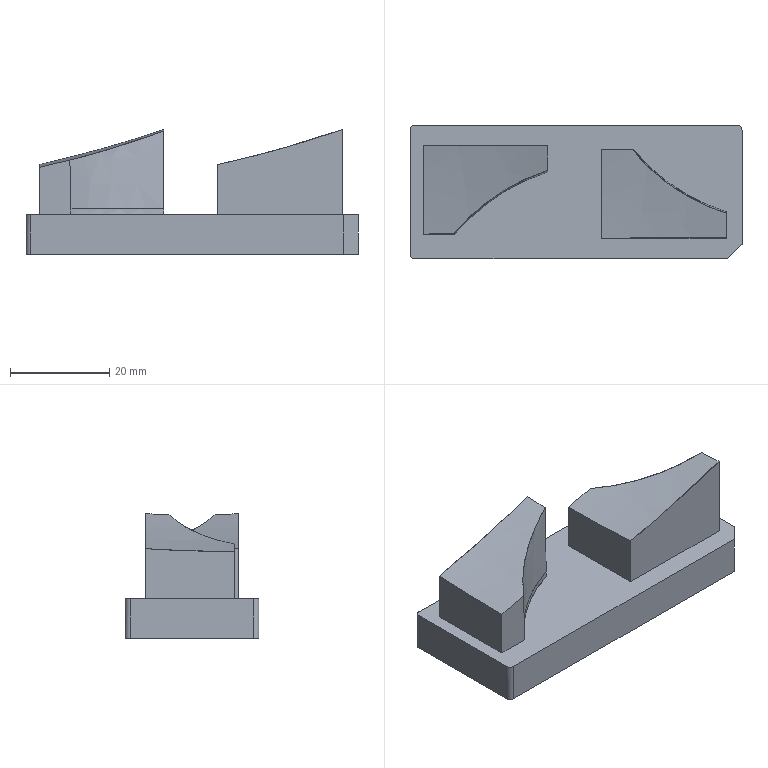NC program | PowerMill | posted with a generic post | part box 67 x 27 x 25.167 mm
Lines 9936 to 10890 of 102458:
N10033 M6
N10034 S18000 M03
N10035 G00 G90 X0.0 Y0.0
N10036 G43 Z9.797 H2
N10037
N10038 G05 P10000 R4
N10039 X-5.4152 Y3.5784
N10040 Z0.7883
N10041 G01 Z-0.4117 F3600.0
N10042 X-5.4161 Y3.6004 F6000.0
N10043 G03 X-5.6216 Y3.7906 I-0.1978 J-0.0077
N10044 G01 X-5.8566 Y3.7814
N10045 X-6.3615 Y3.9044
N10046 X-6.8327 Y4.1332
N10047 X-7.1219 Y4.3925
N10048 X-7.3208 Y4.6168
N10049 X-7.4743 Y4.8805
N10050 X-7.6448 Y5.3686
N10051 X-7.7024 Y5.8566
N10052 X-8.2969 Y8.9999
N10053 X-8.3233 Y9.273
N10054 X-8.2722 Y9.7611
N10055 X-8.0896 Y10.2491
N10056 X-7.725 Y10.7372
N10057 X-7.3208 Y11.0423
N10058 X-6.9004 Y11.2252
N10059 X-6.3447 Y11.3099
N10060 X-5.3686 Y11.2842
N10061 X-5.1132 Y11.2252
N10062 X-4.8805 Y11.139
N10063 X-4.3925 Y10.8322
N10064 X-4.2886 Y10.7372
N10065 X-3.924 Y10.2491
N10066 X-3.7414 Y9.7611
N10067 X-3.6896 Y9.273
N10068 X-3.6899 Y5.8566
N10069 X-3.7357 Y5.3686
N10070 X-3.9016 Y4.8805
N10071 X-4.2608 Y4.3925
N10072 X-4.3925 Y4.253
N10073 X-4.8805 Y3.9455
N10074 X-5.014 Y3.9044
N10075 X-5.2381 Y3.8387
N10076 G00 Z3.5896
N10077 G01 X-2.8266 Y3.5215 F10000.0
N10078 G00 Z0.5896
N10079 G01 Z-0.6104 F3600.0
N10080 X-2.8369 Y3.5409 F6000.0
N10081 G03 X-3.1046 Y3.6229 I-0.1749 J-0.0928
N10082 G01 X-4.1535 Y3.066
N10083 X-4.2516 Y2.9283
N10084 X-4.3925 Y2.7945
N10085 X-4.8805 Y2.4886
N10086 X-4.998 Y2.4403
N10087 X-5.3686 Y2.3172
N10088 X-5.8566 Y2.2169
N10089 X-6.3447 Y2.2398
N10090 X-6.8327 Y2.3884
N10091 X-7.3208 Y2.6994
N10092 X-7.543 Y2.9283
N10093 X-7.8088 Y3.3417
N10094 X-7.9847 Y3.9044
N10095 X-8.3032 Y5.8566
N10096 X-8.3036 Y5.8588
N10097 X-8.7849 Y8.4482
N10098 X-8.9269 Y9.273
N10099 X-8.8758 Y9.7611
N10100 X-8.7849 Y10.0479
N10101 X-8.6931 Y10.2491
N10102 X-8.3286 Y10.7372
N10103 X-7.8088 Y11.1036
N10104 X-7.504 Y11.2252
N10105 X-7.3208 Y11.2711
N10106 X-6.8327 Y11.3101
N10107 X-5.8566
N10108 X-5.3686 Y11.2842
N10109 X-5.1132 Y11.2252
N10110 X-4.8805 Y11.1391
N10111 X-4.3925 Y10.8322
N10112 X-4.2886 Y10.7372
N10113 X-3.924 Y10.2491
N10114 X-3.7414 Y9.7611
N10115 X-3.6896 Y9.273
N10116 X-3.6899 Y4.3925
N10117 X-3.7336 Y3.9044
N10118 X-3.9039 Y3.4164
N10119 X-4.1535 Y3.066
N10120 X-2.8242 Y3.5261 Z-0.8091
N10121 X-2.8346 Y3.5455
N10122 G03 X-3.1027 Y3.6263 I-0.1745 J-0.0936
N10123 G01 X-4.1508 Y3.0641
N10124 X-4.2467 Y2.9283
N10125 X-4.3925 Y2.7908
N10126 X-4.8805 Y2.4842
N10127 X-4.9878 Y2.4403
N10128 X-5.8566 Y2.1507
N10129 X-6.3447 Y2.0339
N10130 X-6.8327 Y2.0366
N10131 X-7.3208 Y2.1646
N10132 X-7.8024 Y2.4403
N10133 X-8.25 Y2.9283
N10134 X-8.481 Y3.4164
N10135 X-8.5847 Y3.9044
N10136 X-8.9074 Y5.8566
N10137 X-9.4613 Y8.7849
N10138 X-9.5304 Y9.273
N10139 X-9.4793 Y9.7611
N10140 X-9.2967 Y10.2491
N10141 X-8.9321 Y10.7372
N10142 X-8.7849 Y10.8677
N10143 X-8.2969 Y11.1564
N10144 X-8.1076 Y11.2252
N10145 X-7.8088 Y11.2903
N10146 X-6.974 Y11.2988
N10147 X-6.9672 Y11.2993
N10148 X-6.8327 Y11.3101
N10149 X-5.8617 Y11.31
N10150 X-5.8566 Y11.3101
N10151 X-5.3686 Y11.2842
N10152 X-5.1132 Y11.2252
N10153 X-4.8805 Y11.1391
N10154 X-4.3925 Y10.8322
N10155 X-4.2886 Y10.7372
N10156 X-3.924 Y10.2491
N10157 X-3.7414 Y9.7611
N10158 X-3.6896 Y9.273
N10159 X-3.6899 Y4.3925
N10160 X-3.7325 Y3.9044
N10161 X-3.9021 Y3.4164
N10162 X-4.1508 Y3.0641
N10163 X-2.8229 Y3.5279 Z-1.0077
N10164 X-2.8333 Y3.5472
N10165 G03 X-3.1016 Y3.6275 I-0.1743 J-0.094
N10166 G01 X-4.1488 Y3.0627
N10167 X-4.2432 Y2.9283
N10168 X-4.3925 Y2.7872
N10169 X-4.8805 Y2.4804
N10170 X-4.9342 Y2.4622
N10171 X-4.9878 Y2.4403
N10172 X-5.8567 Y2.1508
N10173 X-6.4447 Y1.9522
N10174 X-6.8327 Y1.852
N10175 X-7.3208 Y1.8346
N10176 X-7.8088 Y1.9405
N10177 X-8.2969 Y2.1945
N10178 X-8.5828 Y2.4403
N10179 X-8.7849 Y2.689
N10180 X-8.9299 Y2.9283
N10181 X-9.1003 Y3.4164
N10182 X-9.5117 Y5.8566
N10183 X-10.0649 Y8.7849
N10184 X-10.134 Y9.273
N10185 X-10.0829 Y9.7611
N10186 X-9.9003 Y10.2491
N10187 X-9.7611 Y10.4691
N10188 X-9.5357 Y10.7372
N10189 X-9.273 Y10.9512
N10190 X-8.7849 Y11.2013
N10191 X-8.2969 Y11.3032
N10192 X-6.8672 Y11.3072
N10193 X-6.8597 Y11.3079
N10194 X-6.8327 Y11.31
N10195 X-5.8929
N10196 X-5.8566 Y11.3101
N10197 X-5.3686 Y11.2842
N10198 X-5.1132 Y11.2252
N10199 X-4.8805 Y11.1391
N10200 X-4.3925 Y10.8322
N10201 X-4.2886 Y10.7372
N10202 X-3.924 Y10.2491
N10203 X-3.7414 Y9.7611
N10204 X-3.6896 Y9.273
N10205 X-3.6899 Y4.3925
N10206 X-3.7314 Y3.9044
N10207 X-3.9003 Y3.4164
N10208 X-4.1488 Y3.0627
N10209 X-2.8216 Y3.5296 Z-1.2064
N10210 X-2.8321 Y3.549
N10211 G03 X-3.1005 Y3.6286 I-0.174 J-0.0944
N10212 G01 X-4.1468 Y3.0613
N10213 X-4.2398 Y2.9283
N10214 X-4.3925 Y2.7836
N10215 X-4.8805 Y2.4767
N10216 X-4.9811 Y2.4428
N10217 X-4.9845 Y2.4416
N10218 X-4.9878 Y2.4404
N10219 X-5.018 Y2.4303
N10220 X-6.4332 Y1.9522
N10221 X-7.3208 Y1.6489
N10222 X-7.8088 Y1.611
N10223 X-8.2969 Y1.6947
N10224 X-8.7849 Y1.9191
N10225 X-9.273 Y2.3545
N10226 X-9.5969 Y2.9283
N10227 X-9.7102 Y3.4164
N10228 X-10.2931 Y6.8327
N10229 X-10.6685 Y8.7849
N10230 X-10.7376 Y9.273
N10231 X-10.6865 Y9.7611
N10232 X-10.5038 Y10.2491
N10233 X-10.2491 Y10.619
N10234 X-10.1393 Y10.7372
N10235 X-9.7611 Y11.0279
N10236 X-9.3147 Y11.2252
N10237 X-8.7849 Y11.3092
N10238 X-6.835 Y11.3098
N10239 X-6.8327 Y11.31
N10240 X-6.3069 Y11.3099
N10241 X-5.8566 Y11.3101
N10242 X-5.3686 Y11.2842
N10243 X-5.1132 Y11.2252
N10244 X-4.8805 Y11.1391
N10245 X-4.3925 Y10.8322
N10246 X-4.2886 Y10.7372
N10247 X-3.924 Y10.2491
N10248 X-3.7414 Y9.7611
N10249 X-3.6896 Y9.273
N10250 X-3.6899 Y4.3925
N10251 X-3.7305 Y3.9044
N10252 X-3.8985 Y3.4164
N10253 X-4.1468 Y3.0613
N10254 X-2.8223 Y3.5227 Z-1.4051
N10255 X-2.8328 Y3.5421
N10256 G03 X-3.1011 Y3.6223 I-0.1742 J-0.094
N10257 G01 X-4.1442 Y3.0594
N10258 X-4.2363 Y2.9283
N10259 X-4.3925 Y2.7799
N10260 X-4.8805 Y2.4731
N10261 X-6.3447 Y1.9781
N10262 X-7.7529 Y1.4642
N10263 X-8.2969 Y1.3898
N10264 X-8.7849 Y1.4526
N10265 X-9.273 Y1.6486
N10266 X-9.7611 Y2.0326
N10267 X-10.0491 Y2.4403
N10268 X-10.2376 Y2.9283
N10269 X-10.4718 Y4.3925
N10270 X-11.2252 Y8.5768
N10271 X-11.3411 Y9.273
N10272 X-11.29 Y9.7611
N10273 X-11.2252 Y9.9783
N10274 X-11.1074 Y10.2491
N10275 X-10.7372 Y10.7398
N10276 X-10.2491 Y11.0905
N10277 X-9.9183 Y11.2252
N10278 X-9.7611 Y11.2654
N10279 X-9.273 Y11.3101
N10280 X-5.8566
N10281 X-5.3686 Y11.2842
N10282 X-5.1132 Y11.2252
N10283 X-4.8805 Y11.1391
N10284 X-4.3925 Y10.8323
N10285 X-4.2886 Y10.7372
N10286 X-3.924 Y10.2491
N10287 X-3.7414 Y9.7611
N10288 X-3.6896 Y9.273
N10289 X-3.6899 Y4.3925
N10290 X-3.7298 Y3.9044
N10291 X-3.833 Y3.6069
N10292 X-3.8985 Y3.4164
N10293 X-3.9011 Y3.41
N10294 X-3.9035 Y3.4036
N10295 X-3.9044 Y3.4008
N10296 X-4.1442 Y3.0594
N10297 X-2.819 Y3.5332 Z-1.6038
N10298 X-2.8296 Y3.5525
N10299 G03 X-3.0984 Y3.6309 I-0.1736 J-0.0952
N10300 G01 X-4.1428 Y3.0584
N10301 X-4.2329 Y2.9283
N10302 X-4.3925 Y2.7763
N10303 X-4.8805 Y2.4695
N10304 X-6.3447 Y1.9745
N10305 X-7.723 Y1.4642
N10306 X-8.2969 Y1.239
N10307 X-8.7849 Y1.1562
N10308 X-9.273 Y1.1947
N10309 X-9.7611 Y1.3645
N10310 X-9.9377 Y1.4642
N10311 X-10.2491 Y1.7071
N10312 X-10.4695 Y1.9522
N10313 X-10.7392 Y2.4403
N10314 X-10.8583 Y2.9283
N10315 X-11.2359 Y5.3686
N10316 X-11.6829 Y7.8088
N10317 X-11.8862 Y8.7849
N10318 X-11.9574 Y9.273
N10319 X-11.9047 Y9.7611
N10320 X-11.7133 Y10.2574
N10321 X-11.354 Y10.7372
N10322 X-11.2252 Y10.849
N10323 X-10.7372 Y11.1486
N10324 X-10.5292 Y11.2252
N10325 X-10.2491 Y11.2876
N10326 X-9.7611 Y11.3102
N10327 X-5.8566 Y11.3101
N10328 X-5.3686 Y11.2842
N10329 X-5.1132 Y11.2252
N10330 X-4.8805 Y11.1391
N10331 X-4.3925 Y10.8323
N10332 X-4.2886 Y10.7372
N10333 X-3.924 Y10.2491
N10334 X-3.7414 Y9.7611
N10335 X-3.6896 Y9.273
N10336 X-3.6899 Y4.3925
N10337 X-3.7291 Y3.9044
N10338 X-3.8949 Y3.4164
N10339 X-3.8999 Y3.4087
N10340 X-3.9045 Y3.4008
N10341 X-3.988 Y3.2819
N10342 X-4.1428 Y3.0584
N10343 X-2.8177 Y3.535 Z-1.8025
N10344 X-2.8283 Y3.5543
N10345 G03 X-3.0973 Y3.6321 I-0.1734 J-0.0956
N10346 G01 X-4.1407 Y3.0571
N10347 X-4.2295 Y2.9283
N10348 X-4.3925 Y2.7727
N10349 X-4.8805 Y2.4658
N10350 X-6.7452 Y1.8262
N10351 X-6.9556 Y1.7483
N10352 X-6.9571 Y1.7477
N10353 X-8.9375 Y0.9761
N10354 X-9.273 Y0.916
N10355 X-9.7611 Y0.9315
N10356 X-9.9735 Y0.9761
N10357 X-10.2491 Y1.0713
N10358 X-10.7372 Y1.3714
N10359 X-10.8396 Y1.4642
N10360 X-11.214 Y1.9522
N10361 X-11.3999 Y2.4403
N10362 X-11.7816 Y4.8805
N10363 X-12.2013 Y7.2069
N10364 X-12.524 Y8.7849
N10365 X-12.598 Y9.273
N10366 X-12.5456 Y9.7611
N10367 X-12.3632 Y10.2491
N10368 X-12.2013 Y10.4992
N10369 X-11.9954 Y10.7372
N10370 X-11.7133 Y10.9644
N10371 X-11.2252 Y11.2065
N10372 X-10.7372 Y11.3049
N10373 X-8.2969 Y11.3115
N10374 X-5.8566 Y11.3101
N10375 X-5.3686 Y11.2842
N10376 X-5.1132 Y11.2252
N10377 X-4.8805 Y11.1391
N10378 X-4.3925 Y10.8323
N10379 X-4.2886 Y10.7372
N10380 X-3.924 Y10.2491
N10381 X-3.7414 Y9.7611
N10382 X-3.6896 Y9.273
N10383 X-3.6899 Y4.3925
N10384 X-3.7283 Y3.9044
N10385 X-3.8931 Y3.4164
N10386 X-4.1407 Y3.0571
N10387 X-2.8164 Y3.5368 Z-2.0012
N10388 X-2.8271 Y3.556
N10389 G03 X-3.0963 Y3.6333 I-0.1732 J-0.0959
N10390 G01 X-4.1387 Y3.0557
N10391 X-4.2261 Y2.9283
N10392 X-4.3925 Y2.769
N10393 X-4.8805 Y2.4622
N10394 X-6.0058 Y2.0816
N10395 X-7.1247 Y1.6825
N10396 X-7.6417 Y1.481
N10397 X-8.8894 Y0.9761
N10398 X-9.273 Y0.8071
N10399 X-9.7611 Y0.6723
N10400 X-10.2491 Y0.6623
N10401 X-10.7372 Y0.7746
N10402 X-11.2252 Y1.0387
N10403 X-11.652 Y1.4642
N10404 X-11.9172 Y1.9522
N10405 X-12.0444 Y2.4403
N10406 X-12.4195 Y4.8805
N10407 X-12.42 Y4.8834
N10408 X-13.0475 Y8.2969
N10409 X-13.1774 Y8.8416
N10410 X-13.2385 Y9.273
N10411 X-13.1774 Y9.7827
N10412 X-13.004 Y10.2491
N10413 X-12.6894 Y10.6786
N10414 X-12.2013 Y11.0598
N10415 X-11.8123 Y11.2252
N10416 X-11.2252 Y11.3101
N10417 X-5.8566
N10418 X-5.3686 Y11.2842
N10419 X-5.1132 Y11.2252
N10420 X-4.8805 Y11.1391
N10421 X-4.3925 Y10.8323
N10422 X-4.2886 Y10.7372
N10423 X-3.924 Y10.2491
N10424 X-3.7414 Y9.7611
N10425 X-3.6896 Y9.273
N10426 X-3.6899 Y4.3925
N10427 X-3.7276 Y3.9044
N10428 X-3.8913 Y3.4164
N10429 X-4.1387 Y3.0557
N10430 X-2.8152 Y3.5386 Z-2.1999
N10431 X-2.8259 Y3.5578
N10432 G03 X-3.0952 Y3.6344 I-0.173 J-0.0963
N10433 G01 X-4.1367 Y3.0543
N10434 X-4.2227 Y2.9283
N10435 X-4.3925 Y2.7654
N10436 X-4.8805 Y2.4586
N10437 X-6.3759 Y1.9522
N10438 X-7.2773 Y1.6231
N10439 X-7.3944 Y1.5774
N10440 X-7.3956 Y1.577
N10441 X-8.8824 Y0.9761
N10442 X-9.9751 Y0.4881
N10443 X-10.2491 Y0.4138
N10444 X-10.7372 Y0.3765
N10445 X-11.2252 Y0.4625
N10446 X-11.7133 Y0.6862
N10447 X-12.0669 Y0.9761
N10448 X-12.2013 Y1.1293
N10449 X-12.4202 Y1.4642
N10450 X-12.5934 Y1.9522
N10451 X-12.6894 Y2.4699
N10452 X-13.0574 Y4.8805
N10453 X-13.5021 Y7.3208
N10454 X-13.8068 Y8.7849
N10455 X-13.8791 Y9.273
N10456 X-13.8274 Y9.7611
N10457 X-13.6448 Y10.2491
N10458 X-13.2782 Y10.7372
N10459 X-13.1774 Y10.8285
N10460 X-12.6894 Y11.1362
N10461 X-12.4539 Y11.2252
N10462 X-12.2013 Y11.2833
N10463 X-11.7133 Y11.3101
N10464 X-5.8566
N10465 X-5.3686 Y11.2842
N10466 X-5.1132 Y11.2252
N10467 X-4.8805 Y11.1391
N10468 X-4.3925 Y10.8323
N10469 X-4.2886 Y10.7372
N10470 X-3.924 Y10.2491
N10471 X-3.7414 Y9.7611
N10472 X-3.6896 Y9.273
N10473 X-3.6899 Y4.3925
N10474 X-3.7269 Y3.9044
N10475 X-3.8896 Y3.4164
N10476 X-4.1367 Y3.0543
N10477 X-2.8139 Y3.5403 Z-2.3985
N10478 X-2.8247 Y3.5595
N10479 G03 X-3.0942 Y3.6355 I-0.1727 J-0.0967
N10480 G01 X-4.1347 Y3.0529
N10481 X-4.2194 Y2.9283
N10482 X-4.3925 Y2.7618
N10483 X-4.8805 Y2.4549
N10484 X-7.3208 Y1.6035
N10485 X-7.3252 Y1.6017
N10486 X-8.8732 Y0.9761
N10487 X-8.8771 Y0.9743
N10488 X-9.9461 Y0.4881
N10489 X-10.7372 Y0.1578
N10490 X-11.2252 Y0.0944
N10491 X-11.7133 Y0.152
N10492 X-12.2013 Y0.3434
N10493 X-12.4208 Y0.4881
N10494 X-12.6894 Y0.7216
N10495 X-12.8921 Y0.9761
N10496 X-13.1338 Y1.4642
N10497 X-13.2394 Y1.9522
N10498 X-13.698 Y4.8805
N10499 X-14.1443 Y7.3208
N10500 X-14.4481 Y8.7849
N10501 X-14.5197 Y9.273
N10502 X-14.4682 Y9.7611
N10503 X-14.2856 Y10.2491
N10504 X-14.1535 Y10.4603
N10505 X-13.9196 Y10.7372
N10506 X-13.6655 Y10.9479
N10507 X-13.1774 Y11.1971
N10508 X-12.6894 Y11.3025
N10509 X-12.2013 Y11.3101
N10510 X-5.8566
N10511 X-5.3686 Y11.2842
N10512 X-5.1132 Y11.2252
N10513 X-4.8805 Y11.1391
N10514 X-4.3925 Y10.8323
N10515 X-4.2886 Y10.7372
N10516 X-3.924 Y10.2491
N10517 X-3.7414 Y9.7611
N10518 X-3.6896 Y9.273
N10519 X-3.6899 Y4.3925
N10520 X-3.7262 Y3.9044
N10521 X-3.8878 Y3.4164
N10522 X-4.1347 Y3.0529
N10523 X-2.8127 Y3.5421 Z-2.5972
N10524 X-2.8234 Y3.5613
N10525 G03 X-3.0931 Y3.6367 I-0.1726 J-0.0971
N10526 G01 X-4.1327 Y3.0516
N10527 X-4.216 Y2.9283
N10528 X-4.3925 Y2.7581
N10529 X-4.8805 Y2.4513
N10530 X-7.3208 Y1.5998
N10531 X-7.3259 Y1.5977
N10532 X-9.273 Y0.7931
N10533 X-9.2777 Y0.7908
N10534 X-10.9399 Y0.0
N10535 X-11.2252 Y-0.1159
N10536 X-11.7133 Y-0.2082
N10537 X-12.2013 Y-0.1793
N10538 X-12.6894 Y-0.0226
N10539 X-13.1774 Y0.2988
N10540 X-13.3581 Y0.4881
N10541 X-13.6664 Y0.9761
N10542 X-13.8124 Y1.4642
N10543 X-14.2607 Y4.3925
N10544 X-14.7865 Y7.3208
N10545 X-15.1296 Y8.9715
N10546 X-15.1602 Y9.273
N10547 X-15.1091 Y9.7611
N10548 X-14.9264 Y10.2491
N10549 X-14.561 Y10.7372
N10550 X-14.1535 Y11.0445
N10551 X-13.737 Y11.2252
N10552 X-13.1774 Y11.3101
N10553 X-5.8566
N10554 X-5.3686 Y11.2842
N10555 X-5.1132 Y11.2252
N10556 X-4.8805 Y11.1391
N10557 X-4.3925 Y10.8323
N10558 X-4.2886 Y10.7372
N10559 X-3.924 Y10.2491
N10560 X-3.7414 Y9.7611
N10561 X-3.6896 Y9.273
N10562 X-3.6899 Y4.3925
N10563 X-3.7255 Y3.9044
N10564 X-3.8861 Y3.4164
N10565 X-4.1327 Y3.0516
N10566 X-2.8114 Y3.5439 Z-2.7959
N10567 X-2.8222 Y3.5631
N10568 G03 X-3.0921 Y3.6379 I-0.1724 J-0.0975
N10569 G01 X-4.1307 Y3.0502
N10570 X-4.2127 Y2.9283
N10571 X-4.3925 Y2.7545
N10572 X-4.8805 Y2.4477
N10573 X-7.3208 Y1.5961
N10574 X-7.73 Y1.4307
N10575 X-9.0288 Y0.8941
N10576 X-9.7006 Y0.5897
N10577 X-10.9066 Y0.0159
N10578 X-10.908 Y0.0152
N10579 X-11.7133 Y-0.3832
N10580 X-12.0825 Y-0.4881
N10581 X-12.6894 Y-0.5057
N10582 X-13.1774 Y-0.3824
N10583 X-13.6655 Y-0.1041
N10584 X-13.7911 Y0.0
N10585 X-14.1535 Y0.4407
N10586 X-14.3802 Y0.9761
N10587 X-14.8987 Y4.3925
N10588 X-15.1578 Y5.8566
N10589 X-15.7314 Y8.7849
N10590 X-15.8008 Y9.273
N10591 X-15.75 Y9.7611
N10592 X-15.5672 Y10.2491
N10593 X-15.2024 Y10.7372
N10594 X-14.6416 Y11.123
N10595 X-14.3785 Y11.2252
N10596 X-14.1535 Y11.2785
N10597 X-13.6655 Y11.3101
N10598 X-5.8566
N10599 X-5.3686 Y11.2842
N10600 X-5.1132 Y11.2252
N10601 X-4.8805 Y11.1391
N10602 X-4.3925 Y10.8323
N10603 X-4.2886 Y10.7372
N10604 X-3.924 Y10.2491
N10605 X-3.7414 Y9.7611
N10606 X-3.6896 Y9.273
N10607 X-3.6899 Y4.3925
N10608 X-3.7248 Y3.9044
N10609 X-3.8843 Y3.4164
N10610 X-4.1307 Y3.0502
N10611 X-2.8102 Y3.5457 Z-2.9946
N10612 X-2.821 Y3.5648
N10613 G03 X-3.091 Y3.6391 I-0.1721 J-0.0979
N10614 G01 X-4.1287 Y3.0489
N10615 X-4.2094 Y2.9283
N10616 X-4.3925 Y2.7509
N10617 X-4.8805 Y2.444
N10618 X-7.3208 Y1.5924
N10619 X-8.1284 Y1.2661
N10620 X-8.9333 Y0.9336
N10621 X-9.7176 Y0.5799
N10622 X-10.4952 Y0.2116
N10623 X-11.8657 Y-0.4881
N10624 X-12.2013 Y-0.6697
N10625 X-12.6894 Y-0.8274
N10626 X-13.1774 Y-0.8583
N10627 X-13.6655 Y-0.7696
N10628 X-14.1535 Y-0.5365
N10629 X-14.6416 Y-0.0873
N10630 X-14.9524 Y0.4881
N10631 X-15.0533 Y0.9761
N10632 X-15.176 Y1.9522
N10633 X-15.5368 Y4.3925
N10634 X-15.8882 Y6.3447
N10635 X-16.4025 Y8.7849
N10636 X-16.4727 Y9.273
N10637 X-16.4213 Y9.7611
N10638 X-16.2409 Y10.2491
N10639 X-16.1057 Y10.4588
N10640 X-15.8783 Y10.7372
N10641 X-15.6177 Y10.9482
N10642 X-15.1296 Y11.1979
N10643 X-14.6416 Y11.3022
N10644 X-14.1536 Y11.3101
N10645 X-13.6655
N10646 X-5.8566
N10647 X-5.3686 Y11.2842
N10648 X-5.1132 Y11.2252
N10649 X-4.8805 Y11.1391
N10650 X-4.3925 Y10.8323
N10651 X-4.2886 Y10.7372
N10652 X-3.924 Y10.2491
N10653 X-3.7414 Y9.7611
N10654 X-3.6896 Y9.273
N10655 X-3.6899 Y4.3925
N10656 X-3.7241 Y3.9044
N10657 X-3.8826 Y3.4164
N10658 X-4.1287 Y3.0489
N10659 X-2.8089 Y3.5475 Z-3.1933
N10660 X-2.8198 Y3.5666
N10661 G03 X-3.09 Y3.6402 I-0.1719 J-0.0983
N10662 G01 X-4.1267 Y3.0475
N10663 X-4.2061 Y2.9283
N10664 X-4.3925 Y2.7472
N10665 X-4.8819 Y2.4403
N10666 X-7.3208 Y1.5887
N10667 X-8.5629 Y1.0867
N10668 X-8.5636 Y1.0864
N10669 X-8.8863 Y0.953
N10670 X-10.5774 Y0.1697
N10671 X-11.0659 Y-0.0797
N10672 X-12.7462 Y-0.9761
N10673 X-13.1774 Y-1.1409
N10674 X-13.6655 Y-1.2043
N10675 X-14.1535 Y-1.1459
N10676 X-14.5959 Y-0.9761
N10677 X-15.1296 Y-0.5773
N10678 X-15.2075 Y-0.4881
N10679 X-15.5103 Y0.0
N10680 X-15.6177 Y0.3183
N10681 X-16.1057 Y3.7609
N10682 X-16.5938 Y6.5531
N10683 X-17.0864 Y8.7849
N10684 X-17.1565 Y9.273
N10685 X-17.1052 Y9.7611
N10686 X-16.9244 Y10.2491
N10687 X-16.5938 Y10.6982
N10688 X-16.1057 Y11.0701
N10689 X-15.7335 Y11.2252
N10690 X-15.1296 Y11.3101
N10691 X-5.8566
N10692 X-5.3686 Y11.2842
N10693 X-5.1132 Y11.2252
N10694 X-4.8805 Y11.1391
N10695 X-4.3925 Y10.8323
N10696 X-4.2886 Y10.7372
N10697 X-3.924 Y10.2491
N10698 X-3.7414 Y9.7611
N10699 X-3.6896 Y9.273
N10700 X-3.6899 Y4.3925
N10701 X-3.7234 Y3.9044
N10702 X-3.8809 Y3.4164
N10703 X-4.1267 Y3.0475
N10704 X-2.8077 Y3.5493 Z-3.392
N10705 X-2.8186 Y3.5683
N10706 G03 X-3.089 Y3.6414 I-0.1717 J-0.0986
N10707 G01 X-4.1246 Y3.0462
N10708 X-4.2028 Y2.9283
N10709 X-4.3925 Y2.7436
N10710 X-4.8739 Y2.4403
N10711 X-7.3208 Y1.5849
N10712 X-8.8273 Y0.9761
N10713 X-9.8866 Y0.4932
N10714 X-10.935 Y-0.0128
N10715 X-11.066 Y-0.0797
N10716 X-11.6284 Y-0.3797
N10717 X-11.6297 Y-0.3804
N10718 X-13.1774 Y-1.2351
N10719 X-13.6464 Y-1.4642
N10720 X-14.1535 Y-1.5679
N10721 X-14.6416 Y-1.5429
N10722 X-14.9488 Y-1.4642
N10723 X-15.1296 Y-1.3924
N10724 X-15.6177 Y-1.0773
N10725 X-15.7261 Y-0.9761
N10726 X-16.0781 Y-0.4881
N10727 X-16.2521 Y0.0
N10728 X-16.5226 Y1.9522
N10729 X-16.8878 Y4.3925
N10730 X-17.2418 Y6.3447
N10731 X-17.7702 Y8.7849
N10732 X-17.8403 Y9.273
N10733 X-17.789 Y9.7611
N10734 X-17.6078 Y10.2491
N10735 X-17.2456 Y10.7372
N10736 X-17.0818 Y10.878
N10737 X-16.5938 Y11.1621
N10738 X-16.4175 Y11.2252
N10739 X-16.1057 Y11.2918
N10740 X-15.6177 Y11.3101
N10741 X-5.8566
N10742 X-5.3686 Y11.2842
N10743 X-5.1132 Y11.2252
N10744 X-4.8805 Y11.1391
N10745 X-4.3925 Y10.8323
N10746 X-4.2886 Y10.7372
N10747 X-3.924 Y10.2491
N10748 X-3.7414 Y9.7611
N10749 X-3.6896 Y9.273
N10750 X-3.6899 Y4.3925
N10751 X-3.7228 Y3.9044
N10752 X-3.8792 Y3.4164
N10753 X-4.1246 Y3.0462
N10754 X-2.8064 Y3.5511 Z-3.5907
N10755 X-2.8175 Y3.5702
N10756 G03 X-3.0879 Y3.6426 I-0.1714 J-0.0991
N10757 G01 X-4.1226 Y3.0449
N10758 X-4.1996 Y2.9283
N10759 X-4.3925 Y2.74
N10760 X-4.866 Y2.4403
N10761 X-7.3208 Y1.5812
N10762 X-8.8182 Y0.9761
N10763 X-10.002 Y0.4364
N10764 X-10.2879 Y0.3039
N10765 X-10.2912 Y0.3022
N10766 X-11.6082 Y-0.3689
N10767 X-11.6285 Y-0.3797
N10768 X-12.4238 Y-0.8189
N10769 X-14.1535 Y-1.8025
N10770 X-14.6416 Y-1.9379
N10771 X-15.0243 Y-1.9522
N10772 X-15.0942
N10773 X-15.6177 Y-1.8356
N10774 X-16.1057 Y-1.5718
N10775 X-16.2423 Y-1.4642
N10776 X-16.5938 Y-1.0641
N10777 X-16.8551 Y-0.4881
N10778 X-17.5735 Y4.3925
N10779 X-17.9286 Y6.3447
N10780 X-18.4541 Y8.7849
N10781 X-18.5241 Y9.273
N10782 X-18.4728 Y9.7611
N10783 X-18.2913 Y10.2491
N10784 X-18.0579 Y10.5893
N10785 X-17.9293 Y10.7372
N10786 X-17.5699 Y11.0145
N10787 X-17.1016 Y11.2252
N10788 X-16.5938 Y11.3085
N10789 X-15.6541 Y11.3087
N10790 X-15.6177 Y11.31
N10791 X-6.2092 Y11.3101
N10792 X-5.8566
N10793 X-5.3686 Y11.2842
N10794 X-5.1132 Y11.2252
N10795 X-4.8805 Y11.1391
N10796 X-4.3925 Y10.8323
N10797 X-4.2886 Y10.7372
N10798 X-3.924 Y10.2491
N10799 X-3.7414 Y9.7611
N10800 X-3.6896 Y9.273
N10801 X-3.6899 Y4.3925
N10802 X-3.7221 Y3.9044
N10803 X-3.8775 Y3.4164
N10804 X-4.1226 Y3.0449
N10805 X-2.8052 Y3.553 Z-3.7893
N10806 X-2.8163 Y3.572
N10807 G03 X-3.0869 Y3.6438 I-0.1712 J-0.0994
N10808 G01 X-4.1206 Y3.0436
N10809 X-4.1963 Y2.9283
N10810 X-4.3925 Y2.7363
N10811 X-4.858 Y2.4403
N10812 X-7.3208 Y1.5775
N10813 X-8.809 Y0.9761
N10814 X-10.5457 Y0.1726
N10815 X-11.1152 Y-0.1176
N10816 X-12.2506 Y-0.7232
N10817 X-12.4238 Y-0.8188
N10818 X-13.004 Y-1.1487
N10819 X-13.0065 Y-1.1503
N10820 X-14.3238 Y-1.9522
N10821 X-14.6416 Y-2.1466
N10822 X-15.1296 Y-2.3255
N10823 X-15.6177 Y-2.3729
N10824 X-16.1057 Y-2.2995
N10825 X-16.5938 Y-2.0892
N10826 X-16.7941 Y-1.9522
N10827 X-17.0818 Y-1.6783
N10828 X-17.2418 Y-1.4642
N10829 X-17.474 Y-0.9761
N10830 X-17.5699 Y-0.4854
N10831 X-17.6875 Y0.4881
N10832 X-18.1022 Y3.4164
N10833 X-18.546 Y5.9714
N10834 X-19.1379 Y8.7849
N10835 X-19.2078 Y9.273
N10836 X-19.1566 Y9.7611
N10837 X-18.9747 Y10.2491
N10838 X-18.613 Y10.7372
N10839 X-18.0579 Y11.1193
N10840 X-17.7857 Y11.2252
N10841 X-17.5699 Y11.2771
N10842 X-17.0818 Y11.3101
N10843 X-5.8566
N10844 X-5.3686 Y11.2842
N10845 X-5.1132 Y11.2252
N10846 X-4.8805 Y11.1391
N10847 X-4.3925 Y10.8323
N10848 X-4.2886 Y10.7372
N10849 X-3.924 Y10.2491
N10850 X-3.7414 Y9.7611
N10851 X-3.6896 Y9.273
N10852 X-3.6899 Y4.3925
N10853 X-3.7215 Y3.9044
N10854 X-3.8758 Y3.4164
N10855 X-4.1206 Y3.0436
N10856 X-2.804 Y3.5547 Z-3.988
N10857 X-2.8151 Y3.5737
N10858 G03 X-3.0859 Y3.6449 I-0.171 J-0.0998
N10859 G01 X-4.1186 Y3.0422
N10860 X-4.1931 Y2.9283
N10861 X-4.3925 Y2.7327
N10862 X-4.85 Y2.4403
N10863 X-7.3208 Y1.5738
N10864 X-8.7849 Y0.9821
N10865 X-10.6312 Y0.1291
N10866 X-10.9481 Y-0.0324
N10867 X-12.4484 Y-0.8327
N10868 X-13.0041 Y-1.1487
N10869 X-13.8933 Y-1.6901
N10870 X-13.8952 Y-1.6913
N10871 X-15.0646 Y-2.4403
N10872 X-15.6177 Y-2.7109
N10873 X-16.1057 Y-2.7954
N10874 X-16.5938 Y-2.7623
N10875 X-17.0818 Y-2.5977
N10876 X-17.3502 Y-2.4403
N10877 X-17.5699 Y-2.2664
N10878 X-17.8412 Y-1.9522
N10879 X-18.0579 Y-1.5606
N10880 X-18.1979 Y-0.9761
N10881 X-18.4334 Y0.9761
N10882 X-18.7848 Y3.4164
N10883 X-19.2131 Y5.8566
N10884 X-19.7257 Y8.2969
N10885 X-19.8916 Y9.273
N10886 X-19.8405 Y9.7611
N10887 X-19.6582 Y10.2491
N10888 X-19.5221 Y10.4615
N10889 X-19.2967 Y10.7372
N10890 X-19.0341 Y10.9506
N10891 X-18.546 Y11.1993
N10892 X-18.0579 Y11.3029
N10893 X-17.5699 Y11.3102
N10894 X-5.8566 Y11.3101
N10895 X-5.3686 Y11.2842
N10896 X-5.1132 Y11.2252
N10897 X-4.8805 Y11.1391
N10898 X-4.3925 Y10.8323
N10899 X-4.2886 Y10.7372
N10900 X-3.924 Y10.2491
N10901 X-3.7414 Y9.7611
N10902 X-3.6896 Y9.273
N10903 X-3.6899 Y4.3925
N10904 X-3.7208 Y3.9044
N10905 X-3.8741 Y3.4164
N10906 X-4.1186 Y3.0422
N10907 X-2.8028 Y3.5565 Z-4.1867
N10908 X-2.8139 Y3.5755
N10909 G03 X-3.0849 Y3.6461 I-0.1708 J-0.1002
N10910 G01 X-4.1166 Y3.0409
N10911 X-4.1899 Y2.9283
N10912 X-4.3925 Y2.7291
N10913 X-4.842 Y2.4403
N10914 X-6.1943 Y1.9716
N10915 X-7.5402 Y1.4852
N10916 X-8.0406 Y1.283
N10917 X-8.7849 Y0.9784
N10918 X-10.7143 Y0.0868
N10919 X-10.7825 Y0.0521
N10920 X-12.5661 Y-0.8996
N10921 X-12.8188 Y-1.0433
N10922 X-13.8986 Y-1.6934
N10923 X-14.467 Y-2.0574
N10924 X-14.4687 Y-2.0586
N10925 X-15.7635 Y-2.9283
N10926 X-16.1057 Y-3.1078
N10927 X-16.5938 Y-3.2376
N10928 X-17.0818 Y-3.2423
N10929 X-17.5699 Y-3.1258
N10930 X-17.9609 Y-2.9283
N10931 X-18.0579 Y-2.8569
N10932 X-18.4719 Y-2.4403
N10933 X-18.7368 Y-1.9522
N10934 X-18.8509 Y-1.4642
N10935 X-19.1192 Y0.9761
N10936 X-19.5221 Y3.7867
N10937 X-19.8995 Y5.8566
N10938 X-20.4982 Y8.654
N10939 X-20.6036 Y9.273
N10940 X-20.5528 Y9.7611
N10941 X-20.4982 Y9.9498
N10942 X-20.3699 Y10.2491
N10943 X-20.0053 Y10.7372
N10944 X-19.5221 Y11.0864
N10945 X-19.0341 Y11.2633
N10946 X-18.546 Y11.3101
N10947 X-17.5723
N10948 X-17.5699
N10949 X-12.7572
N10950 X-5.8566
N10951 X-5.3686 Y11.2842
N10952 X-5.1132 Y11.2252
N10953 X-4.8805 Y11.1391
N10954 X-4.3925 Y10.8323
N10955 X-4.2886 Y10.7372
N10956 X-3.924 Y10.2491
N10957 X-3.7414 Y9.7611
N10958 X-3.6896 Y9.273
N10959 X-3.6899 Y4.3925
N10960 X-3.7202 Y3.9044
N10961 X-3.8724 Y3.4164
N10962 X-4.1166 Y3.0409
N10963 X-2.8016 Y3.5583 Z-4.3854
N10964 X-2.8128 Y3.5773
N10965 G03 X-3.0839 Y3.6473 I-0.1705 J-0.1006
N10966 G01 X-4.1146 Y3.0396
N10967 X-4.1867 Y2.9283
N10968 X-4.3925 Y2.7254
N10969 X-4.834 Y2.4403
N10970 X-5.3686 Y2.2471
N10971 X-7.5882 Y1.4642
N10972 X-8.7849 Y0.9747
N10973 X-10.7372 Y0.0723
N10974 X-12.6845 Y-0.9669
N10975 X-12.6969 Y-0.9739
N10976 X-13.082 Y-1.2017
N10977 X-13.6509 Y-1.5442
N10978 X-14.7409 Y-2.2414
N10979 X-15.3636 Y-2.6597
N10980 X-15.3654 Y-2.6609
N10981 X-16.4389 Y-3.4164
N10982 X-16.5938 Y-3.506
N10983 X-17.0818 Y-3.684
N10984 X-17.5699 Y-3.7314
N10985 X-18.0579 Y-3.6608
N10986 X-18.546 Y-3.4495
N10987 X-19.0341 Y-3.0377